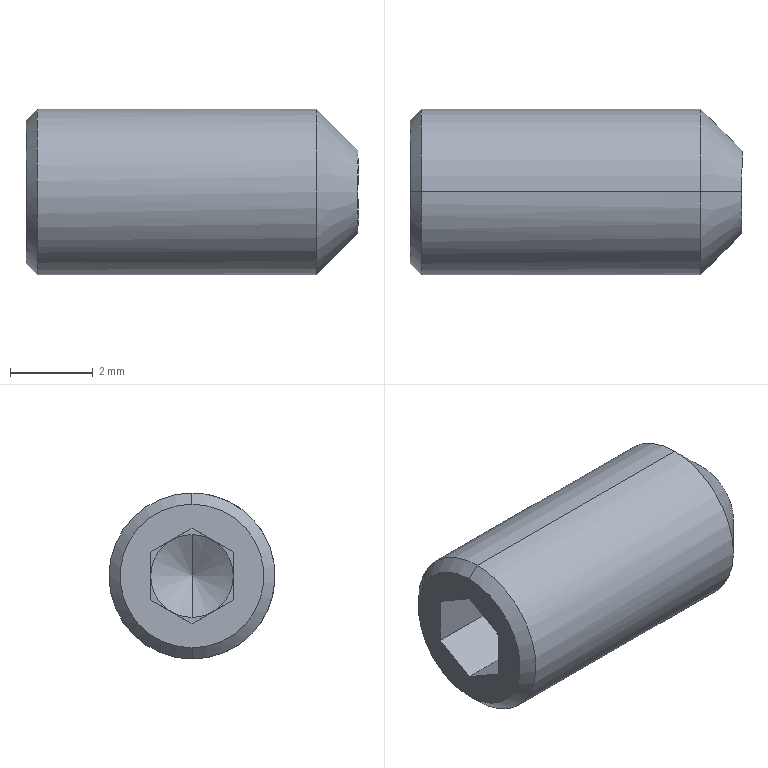Part | STEP file | 103000006212 | 1 solid | 23 faces | box 8 x 4 x 4 mm | volume 88.508 mm3 | plane 13 | cone 8 | cylinder 2 | commonest cylinder face diameters 4 x2
STEP:
#1=CARTESIAN_POINT('',(7.423,0.,0.));
#2=VERTEX_POINT('',#1);
#3=CARTESIAN_POINT('',(8.,1.,0.));
#4=VERTEX_POINT('',#3);
#5=CARTESIAN_POINT('',(250007.711,433013.202,0.));
#6=DIRECTION('',(0.5,0.866,0.));
#7=VECTOR('',#6,1.);
#8=LINE('',#5,#7);
#9=EDGE_CURVE('',#2,#4,#8,.T.);
#10=ORIENTED_EDGE('',*,*,#9,.F.);
#11=CARTESIAN_POINT('',(8.,-1.,0.));
#12=VERTEX_POINT('',#11);
#13=CARTESIAN_POINT('',(250007.711,-433013.202,0.));
#14=DIRECTION('',(0.5,-0.866,0.));
#15=VECTOR('',#14,1.);
#16=LINE('',#13,#15);
#17=EDGE_CURVE('',#2,#12,#16,.T.);
#18=ORIENTED_EDGE('',*,*,#17,.T.);
#19=CARTESIAN_POINT('',(8.,0.,-1.));
#20=VERTEX_POINT('',#19);
#21=CARTESIAN_POINT('',(8.,0.,0.));
#22=DIRECTION('',(1.,0.,0.));
#23=AXIS2_PLACEMENT_3D('',#21,#22,$);
#24=CIRCLE('',#23,1.);
#25=EDGE_CURVE('',#12,#20,#24,.T.);
#26=ORIENTED_EDGE('',*,*,#25,.T.);
#27=CARTESIAN_POINT('',(8.,0.,0.));
#28=DIRECTION('',(1.,0.,0.));
#29=AXIS2_PLACEMENT_3D('',#27,#28,$);
#30=CIRCLE('',#29,1.);
#31=EDGE_CURVE('',#20,#4,#30,.T.);
#32=ORIENTED_EDGE('',*,*,#31,.T.);
#33=EDGE_LOOP('',(#10,#18,#26,#32));
#34=FACE_OUTER_BOUND('',#33,.T.);
#35=CARTESIAN_POINT('',(8.,0.,0.));
#36=DIRECTION('',(1.,0.,0.));
#37=DIRECTION('',(0.,-1.,0.));
#38=AXIS2_PLACEMENT_3D('',#35,#36,#37);
#39=CONICAL_SURFACE('',#38,1.,1.047);
#40=ADVANCED_FACE('',(#34),#39,.F.);
#41=ORIENTED_EDGE('',*,*,#17,.F.);
#42=ORIENTED_EDGE('',*,*,#9,.T.);
#43=CARTESIAN_POINT('',(8.,0.,1.));
#44=VERTEX_POINT('',#43);
#45=CARTESIAN_POINT('',(8.,0.,0.));
#46=DIRECTION('',(1.,0.,0.));
#47=AXIS2_PLACEMENT_3D('',#45,#46,$);
#48=CIRCLE('',#47,1.);
#49=EDGE_CURVE('',#4,#44,#48,.T.);
#50=ORIENTED_EDGE('',*,*,#49,.T.);
#51=CARTESIAN_POINT('',(8.,0.,0.));
#52=DIRECTION('',(1.,0.,0.));
#53=AXIS2_PLACEMENT_3D('',#51,#52,$);
#54=CIRCLE('',#53,1.);
#55=EDGE_CURVE('',#44,#12,#54,.T.);
#56=ORIENTED_EDGE('',*,*,#55,.T.);
#57=EDGE_LOOP('',(#41,#42,#50,#56));
#58=FACE_OUTER_BOUND('',#57,.T.);
#59=CARTESIAN_POINT('',(8.,0.,0.));
#60=DIRECTION('',(1.,0.,0.));
#61=DIRECTION('',(0.,1.,0.));
#62=AXIS2_PLACEMENT_3D('',#59,#60,#61);
#63=CONICAL_SURFACE('',#62,1.,1.047);
#64=ADVANCED_FACE('',(#58),#63,.F.);
#65=CARTESIAN_POINT('',(7.,0.,-2.));
#66=VERTEX_POINT('',#65);
#67=CARTESIAN_POINT('',(-353544.891,0.,-353553.891));
#68=DIRECTION('',(-0.7071,0.,-0.7071));
#69=VECTOR('',#68,1.);
#70=LINE('',#67,#69);
#71=EDGE_CURVE('',#20,#66,#70,.T.);
#72=ORIENTED_EDGE('',*,*,#71,.F.);
#73=ORIENTED_EDGE('',*,*,#25,.F.);
#74=ORIENTED_EDGE('',*,*,#55,.F.);
#75=CARTESIAN_POINT('',(7.,0.,2.));
#76=VERTEX_POINT('',#75);
#77=CARTESIAN_POINT('',(-353544.891,0.,353553.891));
#78=DIRECTION('',(-0.7071,0.,0.7071));
#79=VECTOR('',#78,1.);
#80=LINE('',#77,#79);
#81=EDGE_CURVE('',#44,#76,#80,.T.);
#82=ORIENTED_EDGE('',*,*,#81,.T.);
#83=CARTESIAN_POINT('',(7.,0.,0.));
#84=DIRECTION('',(-1.,0.,0.));
#85=AXIS2_PLACEMENT_3D('',#83,#84,$);
#86=CIRCLE('',#85,2.);
#87=EDGE_CURVE('',#66,#76,#86,.T.);
#88=ORIENTED_EDGE('',*,*,#87,.F.);
#89=EDGE_LOOP('',(#72,#73,#74,#82,#88));
#90=FACE_OUTER_BOUND('',#89,.T.);
#91=CARTESIAN_POINT('',(8.,0.,0.));
#92=DIRECTION('',(-1.,0.,0.));
#93=DIRECTION('',(0.,0.,-1.));
#94=AXIS2_PLACEMENT_3D('',#91,#92,#93);
#95=CONICAL_SURFACE('',#94,1.,0.7854);
#96=ADVANCED_FACE('',(#90),#95,.T.);
#97=ORIENTED_EDGE('',*,*,#31,.F.);
#98=ORIENTED_EDGE('',*,*,#71,.T.);
#99=CARTESIAN_POINT('',(7.,0.,0.));
#100=DIRECTION('',(-1.,0.,0.));
#101=AXIS2_PLACEMENT_3D('',#99,#100,$);
#102=CIRCLE('',#101,2.);
#103=EDGE_CURVE('',#76,#66,#102,.T.);
#104=ORIENTED_EDGE('',*,*,#103,.F.);
#105=ORIENTED_EDGE('',*,*,#81,.F.);
#106=ORIENTED_EDGE('',*,*,#49,.F.);
#107=EDGE_LOOP('',(#97,#98,#104,#105,#106));
#108=FACE_OUTER_BOUND('',#107,.T.);
#109=CARTESIAN_POINT('',(8.,0.,0.));
#110=DIRECTION('',(-1.,0.,0.));
#111=DIRECTION('',(0.,0.,1.));
#112=AXIS2_PLACEMENT_3D('',#109,#110,#111);
#113=CONICAL_SURFACE('',#112,1.,0.7854);
#114=ADVANCED_FACE('',(#108),#113,.T.);
#115=CARTESIAN_POINT('',(0.268,0.,-2.));
#116=VERTEX_POINT('',#115);
#117=CARTESIAN_POINT('',(-0.2621,0.,-2.));
#118=DIRECTION('',(-1.,0.,0.));
#119=VECTOR('',#118,1.);
#120=LINE('',#117,#119);
#121=EDGE_CURVE('',#66,#116,#120,.T.);
#122=ORIENTED_EDGE('',*,*,#121,.F.);
#123=ORIENTED_EDGE('',*,*,#87,.T.);
#124=CARTESIAN_POINT('',(0.268,0.,2.));
#125=VERTEX_POINT('',#124);
#126=CARTESIAN_POINT('',(-0.2621,0.,2.));
#127=DIRECTION('',(-1.,0.,0.));
#128=VECTOR('',#127,1.);
#129=LINE('',#126,#128);
#130=EDGE_CURVE('',#76,#125,#129,.T.);
#131=ORIENTED_EDGE('',*,*,#130,.T.);
#132=CARTESIAN_POINT('',(0.268,0.,-2.));
#133=CARTESIAN_POINT('',(0.268,-0.6283,-2.));
#134=CARTESIAN_POINT('',(0.268,-1.257,-1.753));
#135=CARTESIAN_POINT('',(0.268,-1.753,-1.257));
#136=CARTESIAN_POINT('',(0.268,-2.247,0.));
#137=CARTESIAN_POINT('',(0.268,-1.753,1.257));
#138=CARTESIAN_POINT('',(0.268,-1.257,1.753));
#139=CARTESIAN_POINT('',(0.268,-0.6283,2.));
#140=CARTESIAN_POINT('',(0.268,0.,2.));
#141=B_SPLINE_CURVE_WITH_KNOTS('',5,(#132,#133,#134,#135,#136,#137,#138,#139,#140),.UNSPECIFIED.,.F.,.U.,(6,3,6),(-3.142,0.,3.142),.UNSPECIFIED.);
#142=EDGE_CURVE('',#116,#125,#141,.T.);
#143=ORIENTED_EDGE('',*,*,#142,.F.);
#144=EDGE_LOOP('',(#122,#123,#131,#143));
#145=FACE_OUTER_BOUND('',#144,.T.);
#146=CARTESIAN_POINT('',(-0.2621,0.,0.));
#147=DIRECTION('',(-1.,0.,0.));
#148=DIRECTION('',(0.,0.,-1.));
#149=AXIS2_PLACEMENT_3D('',#146,#147,#148);
#150=CYLINDRICAL_SURFACE('',#149,2.);
#151=ADVANCED_FACE('',(#145),#150,.T.);
#152=ORIENTED_EDGE('',*,*,#103,.T.);
#153=ORIENTED_EDGE('',*,*,#121,.T.);
#154=CARTESIAN_POINT('',(0.268,0.,0.));
#155=DIRECTION('',(-1.,0.,0.));
#156=AXIS2_PLACEMENT_3D('',#154,#155,$);
#157=CIRCLE('',#156,2.);
#158=EDGE_CURVE('',#125,#116,#157,.T.);
#159=ORIENTED_EDGE('',*,*,#158,.F.);
#160=ORIENTED_EDGE('',*,*,#130,.F.);
#161=EDGE_LOOP('',(#152,#153,#159,#160));
#162=FACE_OUTER_BOUND('',#161,.T.);
#163=CARTESIAN_POINT('',(-0.2621,0.,0.));
#164=DIRECTION('',(-1.,0.,0.));
#165=DIRECTION('',(0.,0.,1.));
#166=AXIS2_PLACEMENT_3D('',#163,#164,#165);
#167=CYLINDRICAL_SURFACE('',#166,2.);
#168=ADVANCED_FACE('',(#162),#167,.T.);
#169=CARTESIAN_POINT('',(0.,0.,1.732));
#170=VERTEX_POINT('',#169);
#171=CARTESIAN_POINT('',(353552.659,0.,353554.391));
#172=DIRECTION('',(0.7071,0.,0.7071));
#173=VECTOR('',#172,1.);
#174=LINE('',#171,#173);
#175=EDGE_CURVE('',#170,#125,#174,.T.);
#176=ORIENTED_EDGE('',*,*,#175,.F.);
#177=CARTESIAN_POINT('',(0.,0.,-1.732));
#178=VERTEX_POINT('',#177);
#179=CARTESIAN_POINT('',(0.,0.,0.));
#180=DIRECTION('',(1.,0.,0.));
#181=AXIS2_PLACEMENT_3D('',#179,#180,$);
#182=CIRCLE('',#181,1.732);
#183=EDGE_CURVE('',#178,#170,#182,.F.);
#184=ORIENTED_EDGE('',*,*,#183,.F.);
#185=CARTESIAN_POINT('',(353552.659,0.,-353554.391));
#186=DIRECTION('',(0.7071,0.,-0.7071));
#187=VECTOR('',#186,1.);
#188=LINE('',#185,#187);
#189=EDGE_CURVE('',#178,#116,#188,.T.);
#190=ORIENTED_EDGE('',*,*,#189,.T.);
#191=ORIENTED_EDGE('',*,*,#142,.T.);
#192=EDGE_LOOP('',(#176,#184,#190,#191));
#193=FACE_OUTER_BOUND('',#192,.T.);
#194=CARTESIAN_POINT('',(0.268,0.,0.));
#195=DIRECTION('',(1.,0.,0.));
#196=DIRECTION('',(0.,0.,1.));
#197=AXIS2_PLACEMENT_3D('',#194,#195,#196);
#198=CONICAL_SURFACE('',#197,2.,0.7854);
#199=ADVANCED_FACE('',(#193),#198,.T.);
#200=CARTESIAN_POINT('',(0.,0.,0.));
#201=DIRECTION('',(1.,0.,0.));
#202=AXIS2_PLACEMENT_3D('',#200,#201,$);
#203=CIRCLE('',#202,1.732);
#204=EDGE_CURVE('',#170,#178,#203,.F.);
#205=ORIENTED_EDGE('',*,*,#204,.F.);
#206=ORIENTED_EDGE('',*,*,#175,.T.);
#207=ORIENTED_EDGE('',*,*,#158,.T.);
#208=ORIENTED_EDGE('',*,*,#189,.F.);
#209=EDGE_LOOP('',(#205,#206,#207,#208));
#210=FACE_OUTER_BOUND('',#209,.T.);
#211=CARTESIAN_POINT('',(0.268,0.,0.));
#212=DIRECTION('',(1.,0.,0.));
#213=DIRECTION('',(0.,0.,-1.));
#214=AXIS2_PLACEMENT_3D('',#211,#212,#213);
#215=CONICAL_SURFACE('',#214,2.,0.7854);
#216=ADVANCED_FACE('',(#210),#215,.T.);
#217=ORIENTED_EDGE('',*,*,#183,.T.);
#218=ORIENTED_EDGE('',*,*,#204,.T.);
#219=EDGE_LOOP('',(#217,#218));
#220=FACE_OUTER_BOUND('',#219,.T.);
#221=CARTESIAN_POINT('',(0.,-0.000000001,1.15));
#222=VERTEX_POINT('',#221);
#223=CARTESIAN_POINT('',(0.,0.9959,0.575));
#224=VERTEX_POINT('',#223);
#225=CARTESIAN_POINT('',(0.,0.498,0.8625));
#226=DIRECTION('',(0.,0.866,-0.5));
#227=VECTOR('',#226,1.);
#228=LINE('',#225,#227);
#229=EDGE_CURVE('',#222,#224,#228,.T.);
#230=ORIENTED_EDGE('',*,*,#229,.F.);
#231=CARTESIAN_POINT('',(0.,-0.9959,0.575));
#232=VERTEX_POINT('',#231);
#233=CARTESIAN_POINT('',(0.,-0.498,0.8625));
#234=DIRECTION('',(0.,0.866,0.5));
#235=VECTOR('',#234,1.);
#236=LINE('',#233,#235);
#237=EDGE_CURVE('',#232,#222,#236,.T.);
#238=ORIENTED_EDGE('',*,*,#237,.F.);
#239=CARTESIAN_POINT('',(0.,-0.9959,-0.575));
#240=VERTEX_POINT('',#239);
#241=CARTESIAN_POINT('',(0.,-0.9959,0.));
#242=DIRECTION('',(0.,0.,1.));
#243=VECTOR('',#242,1.);
#244=LINE('',#241,#243);
#245=EDGE_CURVE('',#240,#232,#244,.T.);
#246=ORIENTED_EDGE('',*,*,#245,.F.);
#247=CARTESIAN_POINT('',(0.,-0.000000001,-1.15));
#248=VERTEX_POINT('',#247);
#249=CARTESIAN_POINT('',(0.,-0.498,-0.8625));
#250=DIRECTION('',(0.,-0.866,0.5));
#251=VECTOR('',#250,1.);
#252=LINE('',#249,#251);
#253=EDGE_CURVE('',#248,#240,#252,.T.);
#254=ORIENTED_EDGE('',*,*,#253,.F.);
#255=CARTESIAN_POINT('',(0.,0.9959,-0.575));
#256=VERTEX_POINT('',#255);
#257=CARTESIAN_POINT('',(0.,0.498,-0.8625));
#258=DIRECTION('',(0.,-0.866,-0.5));
#259=VECTOR('',#258,1.);
#260=LINE('',#257,#259);
#261=EDGE_CURVE('',#256,#248,#260,.T.);
#262=ORIENTED_EDGE('',*,*,#261,.F.);
#263=CARTESIAN_POINT('',(0.,0.9959,0.));
#264=DIRECTION('',(0.,0.,-1.));
#265=VECTOR('',#264,1.);
#266=LINE('',#263,#265);
#267=EDGE_CURVE('',#224,#256,#266,.T.);
#268=ORIENTED_EDGE('',*,*,#267,.F.);
#269=EDGE_LOOP('',(#230,#238,#246,#254,#262,#268));
#270=FACE_BOUND('',#269,.T.);
#271=CARTESIAN_POINT('',(0.,1.732,0.));
#272=DIRECTION('',(1.,0.,0.));
#273=DIRECTION('',(0.,0.,-1.));
#274=AXIS2_PLACEMENT_3D('',#271,#272,#273);
#275=PLANE('',#274);
#276=ADVANCED_FACE('',(#220,#270),#275,.F.);
#277=ORIENTED_EDGE('',*,*,#229,.T.);
#278=CARTESIAN_POINT('',(1.5,0.9959,0.575));
#279=VERTEX_POINT('',#278);
#280=CARTESIAN_POINT('',(0.75,0.9959,0.575));
#281=DIRECTION('',(-1.,0.,0.));
#282=VECTOR('',#281,1.);
#283=LINE('',#280,#282);
#284=EDGE_CURVE('',#279,#224,#283,.T.);
#285=ORIENTED_EDGE('',*,*,#284,.F.);
#286=CARTESIAN_POINT('',(1.5,0.498,0.8625));
#287=VERTEX_POINT('',#286);
#288=CARTESIAN_POINT('',(1.5,0.7469,0.7188));
#289=DIRECTION('',(0.,0.866,-0.5));
#290=VECTOR('',#289,1.);
#291=LINE('',#288,#290);
#292=EDGE_CURVE('',#287,#279,#291,.T.);
#293=ORIENTED_EDGE('',*,*,#292,.F.);
#294=CARTESIAN_POINT('',(1.5,0.,1.15));
#295=VERTEX_POINT('',#294);
#296=CARTESIAN_POINT('',(1.5,0.249,1.006));
#297=DIRECTION('',(0.,0.866,-0.5));
#298=VECTOR('',#297,1.);
#299=LINE('',#296,#298);
#300=EDGE_CURVE('',#295,#287,#299,.T.);
#301=ORIENTED_EDGE('',*,*,#300,.F.);
#302=CARTESIAN_POINT('',(0.75,0.,1.15));
#303=DIRECTION('',(-1.,0.,0.));
#304=VECTOR('',#303,1.);
#305=LINE('',#302,#304);
#306=EDGE_CURVE('',#295,#222,#305,.T.);
#307=ORIENTED_EDGE('',*,*,#306,.T.);
#308=EDGE_LOOP('',(#277,#285,#293,#301,#307));
#309=FACE_OUTER_BOUND('',#308,.T.);
#310=CARTESIAN_POINT('',(1.5,0.,1.15));
#311=DIRECTION('',(0.,0.5,0.866));
#312=DIRECTION('',(0.,-0.866,0.5));
#313=AXIS2_PLACEMENT_3D('',#310,#311,#312);
#314=PLANE('',#313);
#315=ADVANCED_FACE('',(#309),#314,.F.);
#316=ORIENTED_EDGE('',*,*,#237,.T.);
#317=ORIENTED_EDGE('',*,*,#306,.F.);
#318=CARTESIAN_POINT('',(1.5,-0.498,0.8625));
#319=VERTEX_POINT('',#318);
#320=CARTESIAN_POINT('',(1.5,-0.249,1.006));
#321=DIRECTION('',(0.,0.866,0.5));
#322=VECTOR('',#321,1.);
#323=LINE('',#320,#322);
#324=EDGE_CURVE('',#319,#295,#323,.T.);
#325=ORIENTED_EDGE('',*,*,#324,.F.);
#326=CARTESIAN_POINT('',(1.5,-0.9959,0.575));
#327=VERTEX_POINT('',#326);
#328=CARTESIAN_POINT('',(1.5,-0.7469,0.7187));
#329=DIRECTION('',(0.,0.866,0.5));
#330=VECTOR('',#329,1.);
#331=LINE('',#328,#330);
#332=EDGE_CURVE('',#327,#319,#331,.T.);
#333=ORIENTED_EDGE('',*,*,#332,.F.);
#334=CARTESIAN_POINT('',(0.75,-0.9959,0.575));
#335=DIRECTION('',(-1.,0.,0.));
#336=VECTOR('',#335,1.);
#337=LINE('',#334,#336);
#338=EDGE_CURVE('',#327,#232,#337,.T.);
#339=ORIENTED_EDGE('',*,*,#338,.T.);
#340=EDGE_LOOP('',(#316,#317,#325,#333,#339));
#341=FACE_OUTER_BOUND('',#340,.T.);
#342=CARTESIAN_POINT('',(1.5,-0.9959,0.575));
#343=DIRECTION('',(0.,-0.5,0.866));
#344=DIRECTION('',(0.,-0.866,-0.5));
#345=AXIS2_PLACEMENT_3D('',#342,#343,#344);
#346=PLANE('',#345);
#347=ADVANCED_FACE('',(#341),#346,.F.);
#348=ORIENTED_EDGE('',*,*,#245,.T.);
#349=ORIENTED_EDGE('',*,*,#338,.F.);
#350=CARTESIAN_POINT('',(1.5,-0.9959,0.));
#351=VERTEX_POINT('',#350);
#352=CARTESIAN_POINT('',(1.5,-0.9959,0.2875));
#353=DIRECTION('',(0.,0.,1.));
#354=VECTOR('',#353,1.);
#355=LINE('',#352,#354);
#356=EDGE_CURVE('',#351,#327,#355,.T.);
#357=ORIENTED_EDGE('',*,*,#356,.F.);
#358=CARTESIAN_POINT('',(1.5,-0.9959,-0.575));
#359=VERTEX_POINT('',#358);
#360=CARTESIAN_POINT('',(1.5,-0.9959,-0.2875));
#361=DIRECTION('',(0.,0.,1.));
#362=VECTOR('',#361,1.);
#363=LINE('',#360,#362);
#364=EDGE_CURVE('',#359,#351,#363,.T.);
#365=ORIENTED_EDGE('',*,*,#364,.F.);
#366=CARTESIAN_POINT('',(0.75,-0.9959,-0.575));
#367=DIRECTION('',(-1.,0.,0.));
#368=VECTOR('',#367,1.);
#369=LINE('',#366,#368);
#370=EDGE_CURVE('',#359,#240,#369,.T.);
#371=ORIENTED_EDGE('',*,*,#370,.T.);
#372=EDGE_LOOP('',(#348,#349,#357,#365,#371));
#373=FACE_OUTER_BOUND('',#372,.T.);
#374=CARTESIAN_POINT('',(1.5,-0.9959,-0.575));
#375=DIRECTION('',(0.,-1.,0.));
#376=DIRECTION('',(0.,0.,-1.));
#377=AXIS2_PLACEMENT_3D('',#374,#375,#376);
#378=PLANE('',#377);
#379=ADVANCED_FACE('',(#373),#378,.F.);
#380=ORIENTED_EDGE('',*,*,#253,.T.);
#381=ORIENTED_EDGE('',*,*,#370,.F.);
#382=CARTESIAN_POINT('',(1.5,-0.498,-0.8625));
#383=VERTEX_POINT('',#382);
#384=CARTESIAN_POINT('',(1.5,-0.7469,-0.7188));
#385=DIRECTION('',(0.,-0.866,0.5));
#386=VECTOR('',#385,1.);
#387=LINE('',#384,#386);
#388=EDGE_CURVE('',#383,#359,#387,.T.);
#389=ORIENTED_EDGE('',*,*,#388,.F.);
#390=CARTESIAN_POINT('',(1.5,-0.000000001,-1.15));
#391=VERTEX_POINT('',#390);
#392=CARTESIAN_POINT('',(1.5,-0.249,-1.006));
#393=DIRECTION('',(0.,-0.866,0.5));
#394=VECTOR('',#393,1.);
#395=LINE('',#392,#394);
#396=EDGE_CURVE('',#391,#383,#395,.T.);
#397=ORIENTED_EDGE('',*,*,#396,.F.);
#398=CARTESIAN_POINT('',(0.75,0.,-1.15));
#399=DIRECTION('',(-1.,0.,0.));
#400=VECTOR('',#399,1.);
#401=LINE('',#398,#400);
#402=EDGE_CURVE('',#391,#248,#401,.T.);
#403=ORIENTED_EDGE('',*,*,#402,.T.);
#404=EDGE_LOOP('',(#380,#381,#389,#397,#403));
#405=FACE_OUTER_BOUND('',#404,.T.);
#406=CARTESIAN_POINT('',(1.5,0.,-1.15));
#407=DIRECTION('',(0.,-0.5,-0.866));
#408=DIRECTION('',(0.,0.866,-0.5));
#409=AXIS2_PLACEMENT_3D('',#406,#407,#408);
#410=PLANE('',#409);
#411=ADVANCED_FACE('',(#405),#410,.F.);
#412=ORIENTED_EDGE('',*,*,#261,.T.);
#413=ORIENTED_EDGE('',*,*,#402,.F.);
#414=CARTESIAN_POINT('',(1.5,0.498,-0.8625));
#415=VERTEX_POINT('',#414);
#416=CARTESIAN_POINT('',(1.5,0.249,-1.006));
#417=DIRECTION('',(0.,-0.866,-0.5));
#418=VECTOR('',#417,1.);
#419=LINE('',#416,#418);
#420=EDGE_CURVE('',#415,#391,#419,.T.);
#421=ORIENTED_EDGE('',*,*,#420,.F.);
#422=CARTESIAN_POINT('',(1.5,0.9959,-0.575));
#423=VERTEX_POINT('',#422);
#424=CARTESIAN_POINT('',(1.5,0.7469,-0.7187));
#425=DIRECTION('',(0.,-0.866,-0.5));
#426=VECTOR('',#425,1.);
#427=LINE('',#424,#426);
#428=EDGE_CURVE('',#423,#415,#427,.T.);
#429=ORIENTED_EDGE('',*,*,#428,.F.);
#430=CARTESIAN_POINT('',(0.75,0.9959,-0.575));
#431=DIRECTION('',(-1.,0.,0.));
#432=VECTOR('',#431,1.);
#433=LINE('',#430,#432);
#434=EDGE_CURVE('',#423,#256,#433,.T.);
#435=ORIENTED_EDGE('',*,*,#434,.T.);
#436=EDGE_LOOP('',(#412,#413,#421,#429,#435));
#437=FACE_OUTER_BOUND('',#436,.T.);
#438=CARTESIAN_POINT('',(1.5,0.9959,-0.575));
#439=DIRECTION('',(0.,0.5,-0.866));
#440=DIRECTION('',(0.,0.866,0.5));
#441=AXIS2_PLACEMENT_3D('',#438,#439,#440);
#442=PLANE('',#441);
#443=ADVANCED_FACE('',(#437),#442,.F.);
#444=ORIENTED_EDGE('',*,*,#267,.T.);
#445=ORIENTED_EDGE('',*,*,#434,.F.);
#446=CARTESIAN_POINT('',(1.5,0.9959,0.));
#447=VERTEX_POINT('',#446);
#448=CARTESIAN_POINT('',(1.5,0.9959,-0.2875));
#449=DIRECTION('',(0.,0.,-1.));
#450=VECTOR('',#449,1.);
#451=LINE('',#448,#450);
#452=EDGE_CURVE('',#447,#423,#451,.T.);
#453=ORIENTED_EDGE('',*,*,#452,.F.);
#454=CARTESIAN_POINT('',(1.5,0.9959,0.2875));
#455=DIRECTION('',(0.,0.,-1.));
#456=VECTOR('',#455,1.);
#457=LINE('',#454,#456);
#458=EDGE_CURVE('',#279,#447,#457,.T.);
#459=ORIENTED_EDGE('',*,*,#458,.F.);
#460=ORIENTED_EDGE('',*,*,#284,.T.);
#461=EDGE_LOOP('',(#444,#445,#453,#459,#460));
#462=FACE_OUTER_BOUND('',#461,.T.);
#463=CARTESIAN_POINT('',(1.5,0.9959,0.575));
#464=DIRECTION('',(0.,1.,0.));
#465=DIRECTION('',(0.,0.,1.));
#466=AXIS2_PLACEMENT_3D('',#463,#464,#465);
#467=PLANE('',#466);
#468=ADVANCED_FACE('',(#462),#467,.F.);
#469=CARTESIAN_POINT('',(1.5,0.000000005,0.000000002));
#470=DIRECTION('',(-1.,0.,0.));
#471=AXIS2_PLACEMENT_3D('',#469,#470,$);
#472=CIRCLE('',#471,0.9959);
#473=EDGE_CURVE('',#287,#447,#472,.T.);
#474=ORIENTED_EDGE('',*,*,#473,.F.);
#475=ORIENTED_EDGE('',*,*,#292,.T.);
#476=ORIENTED_EDGE('',*,*,#458,.T.);
#477=EDGE_LOOP('',(#474,#475,#476));
#478=FACE_OUTER_BOUND('',#477,.T.);
#479=CARTESIAN_POINT('',(1.5,0.9959,1.725));
#480=DIRECTION('',(-1.,0.,0.));
#481=DIRECTION('',(0.,0.,1.));
#482=AXIS2_PLACEMENT_3D('',#479,#480,#481);
#483=PLANE('',#482);
#484=ADVANCED_FACE('',(#478),#483,.T.);
#485=CARTESIAN_POINT('',(1.5,0.,0.9959));
#486=VERTEX_POINT('',#485);
#487=CARTESIAN_POINT('',(1.5,-0.000000002,0.00000001));
#488=DIRECTION('',(-1.,0.,0.));
#489=AXIS2_PLACEMENT_3D('',#487,#488,$);
#490=CIRCLE('',#489,0.9959);
#491=EDGE_CURVE('',#319,#486,#490,.T.);
#492=ORIENTED_EDGE('',*,*,#491,.F.);
#493=ORIENTED_EDGE('',*,*,#324,.T.);
#494=ORIENTED_EDGE('',*,*,#300,.T.);
#495=CARTESIAN_POINT('',(1.5,0.000000003,0.00000001));
#496=DIRECTION('',(-1.,0.,0.));
#497=AXIS2_PLACEMENT_3D('',#495,#496,$);
#498=CIRCLE('',#497,0.9959);
#499=EDGE_CURVE('',#486,#287,#498,.T.);
#500=ORIENTED_EDGE('',*,*,#499,.F.);
#501=EDGE_LOOP('',(#492,#493,#494,#500));
#502=FACE_OUTER_BOUND('',#501,.T.);
#503=CARTESIAN_POINT('',(1.5,0.9959,1.725));
#504=DIRECTION('',(-1.,0.,0.));
#505=DIRECTION('',(0.,0.,1.));
#506=AXIS2_PLACEMENT_3D('',#503,#504,#505);
#507=PLANE('',#506);
#508=ADVANCED_FACE('',(#502),#507,.T.);
#509=CARTESIAN_POINT('',(1.5,-0.000000005,0.000000002));
#510=DIRECTION('',(-1.,0.,0.));
#511=AXIS2_PLACEMENT_3D('',#509,#510,$);
#512=CIRCLE('',#511,0.9959);
#513=EDGE_CURVE('',#351,#319,#512,.T.);
#514=ORIENTED_EDGE('',*,*,#513,.F.);
#515=ORIENTED_EDGE('',*,*,#356,.T.);
#516=ORIENTED_EDGE('',*,*,#332,.T.);
#517=EDGE_LOOP('',(#514,#515,#516));
#518=FACE_OUTER_BOUND('',#517,.T.);
#519=CARTESIAN_POINT('',(1.5,0.9959,1.725));
#520=DIRECTION('',(-1.,0.,0.));
#521=DIRECTION('',(0.,0.,1.));
#522=AXIS2_PLACEMENT_3D('',#519,#520,#521);
#523=PLANE('',#522);
#524=ADVANCED_FACE('',(#518),#523,.T.);
#525=CARTESIAN_POINT('',(1.5,0.000000001,0.));
#526=DIRECTION('',(-1.,0.,0.));
#527=AXIS2_PLACEMENT_3D('',#525,#526,$);
#528=CIRCLE('',#527,0.9959);
#529=EDGE_CURVE('',#383,#351,#528,.T.);
#530=ORIENTED_EDGE('',*,*,#529,.F.);
#531=ORIENTED_EDGE('',*,*,#388,.T.);
#532=ORIENTED_EDGE('',*,*,#364,.T.);
#533=EDGE_LOOP('',(#530,#531,#532));
#534=FACE_OUTER_BOUND('',#533,.T.);
#535=CARTESIAN_POINT('',(1.5,0.9959,1.725));
#536=DIRECTION('',(-1.,0.,0.));
#537=DIRECTION('',(0.,0.,1.));
#538=AXIS2_PLACEMENT_3D('',#535,#536,#537);
#539=PLANE('',#538);
#540=ADVANCED_FACE('',(#534),#539,.T.);
#541=CARTESIAN_POINT('',(1.5,0.,-0.9959));
#542=VERTEX_POINT('',#541);
#543=CARTESIAN_POINT('',(1.5,0.000000003,-0.000000011));
#544=DIRECTION('',(-1.,0.,0.));
#545=AXIS2_PLACEMENT_3D('',#543,#544,$);
#546=CIRCLE('',#545,0.9959);
#547=EDGE_CURVE('',#415,#542,#546,.T.);
#548=ORIENTED_EDGE('',*,*,#547,.F.);
#549=ORIENTED_EDGE('',*,*,#420,.T.);
#550=ORIENTED_EDGE('',*,*,#396,.T.);
#551=CARTESIAN_POINT('',(1.5,-0.000000002,-0.000000011));
#552=DIRECTION('',(-1.,0.,0.));
#553=AXIS2_PLACEMENT_3D('',#551,#552,$);
#554=CIRCLE('',#553,0.9959);
#555=EDGE_CURVE('',#542,#383,#554,.T.);
#556=ORIENTED_EDGE('',*,*,#555,.F.);
#557=EDGE_LOOP('',(#548,#549,#550,#556));
#558=FACE_OUTER_BOUND('',#557,.T.);
#559=CARTESIAN_POINT('',(1.5,0.9959,1.725));
#560=DIRECTION('',(-1.,0.,0.));
#561=DIRECTION('',(0.,0.,1.));
#562=AXIS2_PLACEMENT_3D('',#559,#560,#561);
#563=PLANE('',#562);
#564=ADVANCED_FACE('',(#558),#563,.T.);
#565=CARTESIAN_POINT('',(1.5,-0.000000001,0.));
#566=DIRECTION('',(-1.,0.,0.));
#567=AXIS2_PLACEMENT_3D('',#565,#566,$);
#568=CIRCLE('',#567,0.9959);
#569=EDGE_CURVE('',#447,#415,#568,.T.);
#570=ORIENTED_EDGE('',*,*,#569,.F.);
#571=ORIENTED_EDGE('',*,*,#452,.T.);
#572=ORIENTED_EDGE('',*,*,#428,.T.);
#573=EDGE_LOOP('',(#570,#571,#572));
#574=FACE_OUTER_BOUND('',#573,.T.);
#575=CARTESIAN_POINT('',(1.5,0.9959,1.725));
#576=DIRECTION('',(-1.,0.,0.));
#577=DIRECTION('',(0.,0.,1.));
#578=AXIS2_PLACEMENT_3D('',#575,#576,#577);
#579=PLANE('',#578);
#580=ADVANCED_FACE('',(#574),#579,.T.);
#581=CARTESIAN_POINT('',(2.075,0.,0.));
#582=VERTEX_POINT('',#581);
#583=CARTESIAN_POINT('',(-250497.925,0.,-433878.727));
#584=DIRECTION('',(-0.5,0.,-0.866));
#585=VECTOR('',#584,1.);
#586=LINE('',#583,#585);
#587=EDGE_CURVE('',#582,#542,#586,.T.);
#588=ORIENTED_EDGE('',*,*,#587,.F.);
#589=CARTESIAN_POINT('',(-250497.925,0.,433878.727));
#590=DIRECTION('',(-0.5,0.,0.866));
#591=VECTOR('',#590,1.);
#592=LINE('',#589,#591);
#593=EDGE_CURVE('',#582,#486,#592,.T.);
#594=ORIENTED_EDGE('',*,*,#593,.T.);
#595=ORIENTED_EDGE('',*,*,#499,.T.);
#596=ORIENTED_EDGE('',*,*,#473,.T.);
#597=ORIENTED_EDGE('',*,*,#569,.T.);
#598=ORIENTED_EDGE('',*,*,#547,.T.);
#599=EDGE_LOOP('',(#588,#594,#595,#596,#597,#598));
#600=FACE_OUTER_BOUND('',#599,.T.);
#601=CARTESIAN_POINT('',(-997.925,0.,0.));
#602=DIRECTION('',(-1.,0.,0.));
#603=DIRECTION('',(0.,0.,1.));
#604=AXIS2_PLACEMENT_3D('',#601,#602,#603);
#605=CONICAL_SURFACE('',#604,1732.051,1.047);
#606=ADVANCED_FACE('',(#600),#605,.F.);
#607=ORIENTED_EDGE('',*,*,#593,.F.);
#608=ORIENTED_EDGE('',*,*,#587,.T.);
#609=ORIENTED_EDGE('',*,*,#555,.T.);
#610=ORIENTED_EDGE('',*,*,#529,.T.);
#611=ORIENTED_EDGE('',*,*,#513,.T.);
#612=ORIENTED_EDGE('',*,*,#491,.T.);
#613=EDGE_LOOP('',(#607,#608,#609,#610,#611,#612));
#614=FACE_OUTER_BOUND('',#613,.T.);
#615=CARTESIAN_POINT('',(-997.925,0.,0.));
#616=DIRECTION('',(-1.,0.,0.));
#617=DIRECTION('',(0.,0.,-1.));
#618=AXIS2_PLACEMENT_3D('',#615,#616,#617);
#619=CONICAL_SURFACE('',#618,1732.051,1.047);
#620=ADVANCED_FACE('',(#614),#619,.F.);
#621=CLOSED_SHELL('',(#40,#64,#96,#114,#151,#168,#199,#216,#276,#315,#347,#379,#411,#443,#468,#484,#508,#524,#540,#564,#580,#606,#620));
#622=MANIFOLD_SOLID_BREP('',#621);
#623=(LENGTH_UNIT()NAMED_UNIT(*)SI_UNIT(.MILLI.,.METRE.));
#624=UNCERTAINTY_MEASURE_WITH_UNIT(LENGTH_MEASURE(0.005),#623,'','');
#625=(NAMED_UNIT(*)PLANE_ANGLE_UNIT()SI_UNIT($,.RADIAN.));
#626=(NAMED_UNIT(*)SI_UNIT($,.STERADIAN.)SOLID_ANGLE_UNIT());
#627=(GEOMETRIC_REPRESENTATION_CONTEXT(3)GLOBAL_UNCERTAINTY_ASSIGNED_CONTEXT((#624))GLOBAL_UNIT_ASSIGNED_CONTEXT((#623,#625,#626))REPRESENTATION_CONTEXT('',''));
#628=ADVANCED_BREP_SHAPE_REPRESENTATION('',(#622),#627);